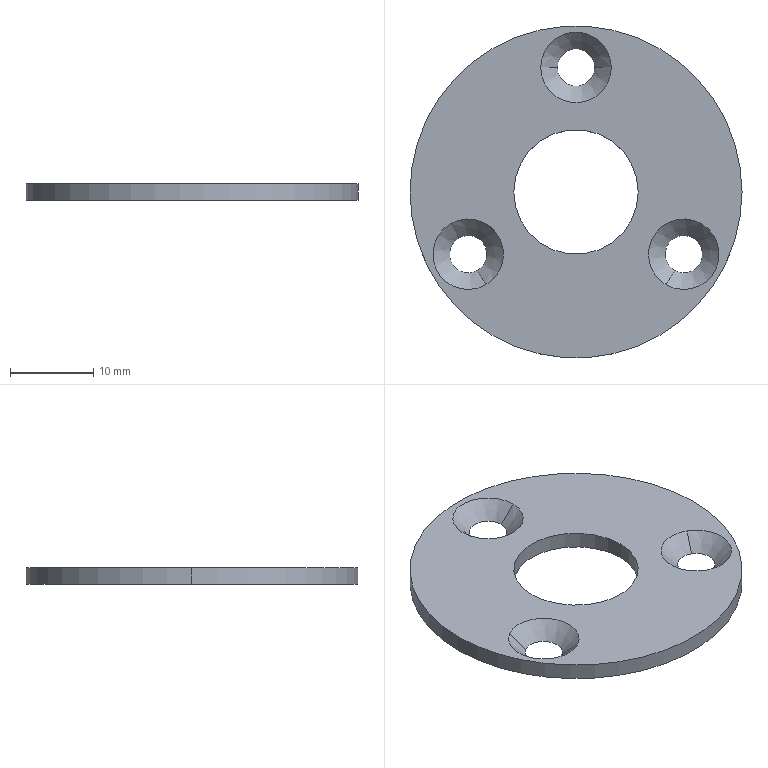Part | SolidWorks | features CirPattern 1, RevCut 1, Revolution 1 | 1 solid | 12 faces | box 40 x 40 x 2 mm | volume 1954 mm3 | cone 6 | cylinder 4 | plane 2 | commonest cylinder face diameters 15 x2 40 x2
STEP:
#1=CARTESIAN_POINT('',(-11.865,-9.449,-2.));
#2=VERTEX_POINT('',#1);
#3=CARTESIAN_POINT('',(-14.115,-5.551,-2.));
#4=VERTEX_POINT('',#3);
#5=CARTESIAN_POINT('',(-12.99,-7.5,-2.));
#6=DIRECTION('',(0.,0.,1.));
#7=DIRECTION('',(-0.5,0.866,0.));
#8=AXIS2_PLACEMENT_3D('',#5,#6,#7);
#9=CIRCLE('',#8,2.25);
#10=EDGE_CURVE('',#2,#4,#9,.T.);
#11=ORIENTED_EDGE('',*,*,#10,.F.);
#12=CARTESIAN_POINT('',(-10.865,-11.181,0.));
#13=VERTEX_POINT('',#12);
#14=CARTESIAN_POINT('',(-11.865,-9.449,-2.));
#15=DIRECTION('',(0.3536,-0.6124,0.7071));
#16=VECTOR('',#15,1000.);
#17=LINE('',#14,#16);
#18=EDGE_CURVE('',#2,#13,#17,.T.);
#19=ORIENTED_EDGE('',*,*,#18,.T.);
#20=CARTESIAN_POINT('',(-15.115,-3.819,0.));
#21=VERTEX_POINT('',#20);
#22=CARTESIAN_POINT('',(-12.99,-7.5,0.));
#23=DIRECTION('',(0.,0.,1.));
#24=DIRECTION('',(-0.5,0.866,0.));
#25=AXIS2_PLACEMENT_3D('',#22,#23,#24);
#26=CIRCLE('',#25,4.25);
#27=EDGE_CURVE('',#13,#21,#26,.T.);
#28=ORIENTED_EDGE('',*,*,#27,.T.);
#29=CARTESIAN_POINT('',(-14.115,-5.551,-2.));
#30=DIRECTION('',(-0.3536,0.6124,0.7071));
#31=VECTOR('',#30,1000.);
#32=LINE('',#29,#31);
#33=EDGE_CURVE('',#4,#21,#32,.T.);
#34=ORIENTED_EDGE('',*,*,#33,.F.);
#35=EDGE_LOOP('',(#11,#19,#28,#34));
#36=FACE_OUTER_BOUND('',#35,.T.);
#37=CARTESIAN_POINT('',(-12.99,-7.5,-2.));
#38=DIRECTION('',(0.,0.,1.));
#39=DIRECTION('',(-0.5,0.866,0.));
#40=AXIS2_PLACEMENT_3D('',#37,#38,#39);
#41=CONICAL_SURFACE('',#40,2.25,0.7854);
#42=ADVANCED_FACE('',(#36),#41,.F.);
#43=CARTESIAN_POINT('',(14.115,-5.551,-2.));
#44=VERTEX_POINT('',#43);
#45=CARTESIAN_POINT('',(11.865,-9.449,-2.));
#46=VERTEX_POINT('',#45);
#47=CARTESIAN_POINT('',(12.99,-7.5,-2.));
#48=DIRECTION('',(0.,0.,1.));
#49=DIRECTION('',(-0.5,-0.866,0.));
#50=AXIS2_PLACEMENT_3D('',#47,#48,#49);
#51=CIRCLE('',#50,2.25);
#52=EDGE_CURVE('',#44,#46,#51,.T.);
#53=ORIENTED_EDGE('',*,*,#52,.F.);
#54=CARTESIAN_POINT('',(15.115,-3.819,0.));
#55=VERTEX_POINT('',#54);
#56=CARTESIAN_POINT('',(14.115,-5.551,-2.));
#57=DIRECTION('',(0.3536,0.6124,0.7071));
#58=VECTOR('',#57,1000.);
#59=LINE('',#56,#58);
#60=EDGE_CURVE('',#44,#55,#59,.T.);
#61=ORIENTED_EDGE('',*,*,#60,.T.);
#62=CARTESIAN_POINT('',(10.865,-11.181,0.));
#63=VERTEX_POINT('',#62);
#64=CARTESIAN_POINT('',(12.99,-7.5,0.));
#65=DIRECTION('',(0.,0.,1.));
#66=DIRECTION('',(-0.5,-0.866,0.));
#67=AXIS2_PLACEMENT_3D('',#64,#65,#66);
#68=CIRCLE('',#67,4.25);
#69=EDGE_CURVE('',#55,#63,#68,.T.);
#70=ORIENTED_EDGE('',*,*,#69,.T.);
#71=CARTESIAN_POINT('',(11.865,-9.449,-2.));
#72=DIRECTION('',(-0.3536,-0.6124,0.7071));
#73=VECTOR('',#72,1000.);
#74=LINE('',#71,#73);
#75=EDGE_CURVE('',#46,#63,#74,.T.);
#76=ORIENTED_EDGE('',*,*,#75,.F.);
#77=EDGE_LOOP('',(#53,#61,#70,#76));
#78=FACE_OUTER_BOUND('',#77,.T.);
#79=CARTESIAN_POINT('',(12.99,-7.5,-2.));
#80=DIRECTION('',(0.,0.,1.));
#81=DIRECTION('',(-0.5,-0.866,0.));
#82=AXIS2_PLACEMENT_3D('',#79,#80,#81);
#83=CONICAL_SURFACE('',#82,2.25,0.7854);
#84=ADVANCED_FACE('',(#78),#83,.F.);
#85=CARTESIAN_POINT('',(-2.25,15.,-2.));
#86=VERTEX_POINT('',#85);
#87=CARTESIAN_POINT('',(2.25,15.,-2.));
#88=VERTEX_POINT('',#87);
#89=CARTESIAN_POINT('',(0.,15.,-2.));
#90=DIRECTION('',(0.,0.,1.));
#91=DIRECTION('',(1.,0.,0.));
#92=AXIS2_PLACEMENT_3D('',#89,#90,#91);
#93=CIRCLE('',#92,2.25);
#94=EDGE_CURVE('',#86,#88,#93,.T.);
#95=ORIENTED_EDGE('',*,*,#94,.F.);
#96=CARTESIAN_POINT('',(-4.25,15.,0.));
#97=VERTEX_POINT('',#96);
#98=CARTESIAN_POINT('',(-2.25,15.,-2.));
#99=DIRECTION('',(-0.7071,0.,0.7071));
#100=VECTOR('',#99,1000.);
#101=LINE('',#98,#100);
#102=EDGE_CURVE('',#86,#97,#101,.T.);
#103=ORIENTED_EDGE('',*,*,#102,.T.);
#104=CARTESIAN_POINT('',(4.25,15.,0.));
#105=VERTEX_POINT('',#104);
#106=CARTESIAN_POINT('',(0.,15.,0.));
#107=DIRECTION('',(0.,0.,1.));
#108=DIRECTION('',(1.,0.,0.));
#109=AXIS2_PLACEMENT_3D('',#106,#107,#108);
#110=CIRCLE('',#109,4.25);
#111=EDGE_CURVE('',#97,#105,#110,.T.);
#112=ORIENTED_EDGE('',*,*,#111,.T.);
#113=CARTESIAN_POINT('',(2.25,15.,-2.));
#114=DIRECTION('',(0.7071,0.,0.7071));
#115=VECTOR('',#114,1000.);
#116=LINE('',#113,#115);
#117=EDGE_CURVE('',#88,#105,#116,.T.);
#118=ORIENTED_EDGE('',*,*,#117,.F.);
#119=EDGE_LOOP('',(#95,#103,#112,#118));
#120=FACE_OUTER_BOUND('',#119,.T.);
#121=CARTESIAN_POINT('',(0.,15.,-2.));
#122=DIRECTION('',(0.,0.,1.));
#123=DIRECTION('',(1.,0.,0.));
#124=AXIS2_PLACEMENT_3D('',#121,#122,#123);
#125=CONICAL_SURFACE('',#124,2.25,0.7854);
#126=ADVANCED_FACE('',(#120),#125,.F.);
#127=CARTESIAN_POINT('',(-7.5,0.,-2.));
#128=VERTEX_POINT('',#127);
#129=CARTESIAN_POINT('',(7.5,0.,-2.));
#130=VERTEX_POINT('',#129);
#131=CARTESIAN_POINT('',(0.,0.,-2.));
#132=DIRECTION('',(0.,0.,1.));
#133=DIRECTION('',(1.,0.,0.));
#134=AXIS2_PLACEMENT_3D('',#131,#132,#133);
#135=CIRCLE('',#134,7.5);
#136=EDGE_CURVE('',#128,#130,#135,.T.);
#137=ORIENTED_EDGE('',*,*,#136,.F.);
#138=CARTESIAN_POINT('',(-7.5,0.,0.));
#139=VERTEX_POINT('',#138);
#140=CARTESIAN_POINT('',(-7.5,0.,4.367));
#141=DIRECTION('',(0.,0.,1.));
#142=VECTOR('',#141,1000.);
#143=LINE('',#140,#142);
#144=EDGE_CURVE('',#128,#139,#143,.T.);
#145=ORIENTED_EDGE('',*,*,#144,.T.);
#146=CARTESIAN_POINT('',(7.5,0.,0.));
#147=VERTEX_POINT('',#146);
#148=CARTESIAN_POINT('',(0.,0.,0.));
#149=DIRECTION('',(0.,0.,1.));
#150=DIRECTION('',(1.,0.,0.));
#151=AXIS2_PLACEMENT_3D('',#148,#149,#150);
#152=CIRCLE('',#151,7.5);
#153=EDGE_CURVE('',#139,#147,#152,.T.);
#154=ORIENTED_EDGE('',*,*,#153,.T.);
#155=CARTESIAN_POINT('',(7.5,0.,4.367));
#156=DIRECTION('',(0.,0.,1.));
#157=VECTOR('',#156,1000.);
#158=LINE('',#155,#157);
#159=EDGE_CURVE('',#130,#147,#158,.T.);
#160=ORIENTED_EDGE('',*,*,#159,.F.);
#161=EDGE_LOOP('',(#137,#145,#154,#160));
#162=FACE_OUTER_BOUND('',#161,.T.);
#163=CARTESIAN_POINT('',(0.,0.,4.367));
#164=DIRECTION('',(0.,0.,1.));
#165=DIRECTION('',(1.,0.,0.));
#166=AXIS2_PLACEMENT_3D('',#163,#164,#165);
#167=CYLINDRICAL_SURFACE('',#166,7.5);
#168=ADVANCED_FACE('',(#162),#167,.F.);
#169=CARTESIAN_POINT('',(20.,0.,-2.));
#170=VERTEX_POINT('',#169);
#171=CARTESIAN_POINT('',(-20.,0.,-2.));
#172=VERTEX_POINT('',#171);
#173=CARTESIAN_POINT('',(0.,0.,-2.));
#174=DIRECTION('',(0.,0.,1.));
#175=DIRECTION('',(1.,0.,0.));
#176=AXIS2_PLACEMENT_3D('',#173,#174,#175);
#177=CIRCLE('',#176,20.);
#178=EDGE_CURVE('',#170,#172,#177,.T.);
#179=ORIENTED_EDGE('',*,*,#178,.T.);
#180=CARTESIAN_POINT('',(-20.,0.,0.));
#181=VERTEX_POINT('',#180);
#182=CARTESIAN_POINT('',(-20.,0.,4.367));
#183=DIRECTION('',(0.,0.,1.));
#184=VECTOR('',#183,1000.);
#185=LINE('',#182,#184);
#186=EDGE_CURVE('',#172,#181,#185,.T.);
#187=ORIENTED_EDGE('',*,*,#186,.T.);
#188=CARTESIAN_POINT('',(20.,0.,0.));
#189=VERTEX_POINT('',#188);
#190=CARTESIAN_POINT('',(0.,0.,0.));
#191=DIRECTION('',(0.,0.,1.));
#192=DIRECTION('',(1.,0.,0.));
#193=AXIS2_PLACEMENT_3D('',#190,#191,#192);
#194=CIRCLE('',#193,20.);
#195=EDGE_CURVE('',#189,#181,#194,.T.);
#196=ORIENTED_EDGE('',*,*,#195,.F.);
#197=CARTESIAN_POINT('',(20.,0.,4.367));
#198=DIRECTION('',(0.,0.,1.));
#199=VECTOR('',#198,1000.);
#200=LINE('',#197,#199);
#201=EDGE_CURVE('',#170,#189,#200,.T.);
#202=ORIENTED_EDGE('',*,*,#201,.F.);
#203=EDGE_LOOP('',(#179,#187,#196,#202));
#204=FACE_OUTER_BOUND('',#203,.T.);
#205=CARTESIAN_POINT('',(0.,0.,4.367));
#206=DIRECTION('',(0.,0.,1.));
#207=DIRECTION('',(1.,0.,0.));
#208=AXIS2_PLACEMENT_3D('',#205,#206,#207);
#209=CYLINDRICAL_SURFACE('',#208,20.);
#210=ADVANCED_FACE('',(#204),#209,.T.);
#211=ORIENTED_EDGE('',*,*,#186,.F.);
#212=CARTESIAN_POINT('',(0.,0.,-2.));
#213=DIRECTION('',(0.,0.,1.));
#214=DIRECTION('',(1.,0.,0.));
#215=AXIS2_PLACEMENT_3D('',#212,#213,#214);
#216=CIRCLE('',#215,20.);
#217=EDGE_CURVE('',#172,#170,#216,.T.);
#218=ORIENTED_EDGE('',*,*,#217,.T.);
#219=ORIENTED_EDGE('',*,*,#201,.T.);
#220=CARTESIAN_POINT('',(0.,0.,0.));
#221=DIRECTION('',(0.,0.,1.));
#222=DIRECTION('',(1.,0.,0.));
#223=AXIS2_PLACEMENT_3D('',#220,#221,#222);
#224=CIRCLE('',#223,20.);
#225=EDGE_CURVE('',#181,#189,#224,.T.);
#226=ORIENTED_EDGE('',*,*,#225,.F.);
#227=EDGE_LOOP('',(#211,#218,#219,#226));
#228=FACE_OUTER_BOUND('',#227,.T.);
#229=CARTESIAN_POINT('',(0.,0.,4.367));
#230=DIRECTION('',(0.,0.,1.));
#231=DIRECTION('',(1.,0.,0.));
#232=AXIS2_PLACEMENT_3D('',#229,#230,#231);
#233=CYLINDRICAL_SURFACE('',#232,20.);
#234=ADVANCED_FACE('',(#228),#233,.T.);
#235=CARTESIAN_POINT('',(-12.99,-7.5,0.));
#236=DIRECTION('',(0.,0.,1.));
#237=DIRECTION('',(-0.5,0.866,0.));
#238=AXIS2_PLACEMENT_3D('',#235,#236,#237);
#239=CIRCLE('',#238,4.25);
#240=EDGE_CURVE('',#21,#13,#239,.T.);
#241=ORIENTED_EDGE('',*,*,#240,.F.);
#242=ORIENTED_EDGE('',*,*,#27,.F.);
#243=EDGE_LOOP('',(#241,#242));
#244=FACE_BOUND('',#243,.T.);
#245=CARTESIAN_POINT('',(12.99,-7.5,0.));
#246=DIRECTION('',(0.,0.,1.));
#247=DIRECTION('',(-0.5,-0.866,0.));
#248=AXIS2_PLACEMENT_3D('',#245,#246,#247);
#249=CIRCLE('',#248,4.25);
#250=EDGE_CURVE('',#63,#55,#249,.T.);
#251=ORIENTED_EDGE('',*,*,#250,.F.);
#252=ORIENTED_EDGE('',*,*,#69,.F.);
#253=EDGE_LOOP('',(#251,#252));
#254=FACE_BOUND('',#253,.T.);
#255=CARTESIAN_POINT('',(0.,15.,0.));
#256=DIRECTION('',(0.,0.,1.));
#257=DIRECTION('',(1.,0.,0.));
#258=AXIS2_PLACEMENT_3D('',#255,#256,#257);
#259=CIRCLE('',#258,4.25);
#260=EDGE_CURVE('',#105,#97,#259,.T.);
#261=ORIENTED_EDGE('',*,*,#260,.F.);
#262=ORIENTED_EDGE('',*,*,#111,.F.);
#263=EDGE_LOOP('',(#261,#262));
#264=FACE_BOUND('',#263,.T.);
#265=CARTESIAN_POINT('',(0.,0.,0.));
#266=DIRECTION('',(0.,0.,1.));
#267=DIRECTION('',(1.,0.,0.));
#268=AXIS2_PLACEMENT_3D('',#265,#266,#267);
#269=CIRCLE('',#268,7.5);
#270=EDGE_CURVE('',#147,#139,#269,.T.);
#271=ORIENTED_EDGE('',*,*,#270,.F.);
#272=ORIENTED_EDGE('',*,*,#153,.F.);
#273=EDGE_LOOP('',(#271,#272));
#274=FACE_BOUND('',#273,.T.);
#275=ORIENTED_EDGE('',*,*,#195,.T.);
#276=ORIENTED_EDGE('',*,*,#225,.T.);
#277=EDGE_LOOP('',(#275,#276));
#278=FACE_OUTER_BOUND('',#277,.T.);
#279=CARTESIAN_POINT('',(0.,20.,0.));
#280=DIRECTION('',(0.,0.,-1.));
#281=DIRECTION('',(-1.,0.,0.));
#282=AXIS2_PLACEMENT_3D('',#279,#280,#281);
#283=PLANE('',#282);
#284=ADVANCED_FACE('',(#244,#254,#264,#274,#278),#283,.F.);
#285=ORIENTED_EDGE('',*,*,#144,.F.);
#286=CARTESIAN_POINT('',(0.,0.,-2.));
#287=DIRECTION('',(0.,0.,1.));
#288=DIRECTION('',(1.,0.,0.));
#289=AXIS2_PLACEMENT_3D('',#286,#287,#288);
#290=CIRCLE('',#289,7.5);
#291=EDGE_CURVE('',#130,#128,#290,.T.);
#292=ORIENTED_EDGE('',*,*,#291,.F.);
#293=ORIENTED_EDGE('',*,*,#159,.T.);
#294=ORIENTED_EDGE('',*,*,#270,.T.);
#295=EDGE_LOOP('',(#285,#292,#293,#294));
#296=FACE_OUTER_BOUND('',#295,.T.);
#297=CARTESIAN_POINT('',(0.,0.,4.367));
#298=DIRECTION('',(0.,0.,1.));
#299=DIRECTION('',(1.,0.,0.));
#300=AXIS2_PLACEMENT_3D('',#297,#298,#299);
#301=CYLINDRICAL_SURFACE('',#300,7.5);
#302=ADVANCED_FACE('',(#296),#301,.F.);
#303=CARTESIAN_POINT('',(-12.99,-7.5,-2.));
#304=DIRECTION('',(0.,0.,1.));
#305=DIRECTION('',(-0.5,0.866,0.));
#306=AXIS2_PLACEMENT_3D('',#303,#304,#305);
#307=CIRCLE('',#306,2.25);
#308=EDGE_CURVE('',#4,#2,#307,.T.);
#309=ORIENTED_EDGE('',*,*,#308,.T.);
#310=ORIENTED_EDGE('',*,*,#10,.T.);
#311=EDGE_LOOP('',(#309,#310));
#312=FACE_BOUND('',#311,.T.);
#313=CARTESIAN_POINT('',(12.99,-7.5,-2.));
#314=DIRECTION('',(0.,0.,1.));
#315=DIRECTION('',(-0.5,-0.866,0.));
#316=AXIS2_PLACEMENT_3D('',#313,#314,#315);
#317=CIRCLE('',#316,2.25);
#318=EDGE_CURVE('',#46,#44,#317,.T.);
#319=ORIENTED_EDGE('',*,*,#318,.T.);
#320=ORIENTED_EDGE('',*,*,#52,.T.);
#321=EDGE_LOOP('',(#319,#320));
#322=FACE_BOUND('',#321,.T.);
#323=CARTESIAN_POINT('',(0.,15.,-2.));
#324=DIRECTION('',(0.,0.,1.));
#325=DIRECTION('',(1.,0.,0.));
#326=AXIS2_PLACEMENT_3D('',#323,#324,#325);
#327=CIRCLE('',#326,2.25);
#328=EDGE_CURVE('',#88,#86,#327,.T.);
#329=ORIENTED_EDGE('',*,*,#328,.T.);
#330=ORIENTED_EDGE('',*,*,#94,.T.);
#331=EDGE_LOOP('',(#329,#330));
#332=FACE_BOUND('',#331,.T.);
#333=ORIENTED_EDGE('',*,*,#178,.F.);
#334=ORIENTED_EDGE('',*,*,#217,.F.);
#335=EDGE_LOOP('',(#333,#334));
#336=FACE_OUTER_BOUND('',#335,.T.);
#337=ORIENTED_EDGE('',*,*,#291,.T.);
#338=ORIENTED_EDGE('',*,*,#136,.T.);
#339=EDGE_LOOP('',(#337,#338));
#340=FACE_BOUND('',#339,.T.);
#341=CARTESIAN_POINT('',(0.,7.5,-2.));
#342=DIRECTION('',(0.,0.,1.));
#343=DIRECTION('',(1.,0.,0.));
#344=AXIS2_PLACEMENT_3D('',#341,#342,#343);
#345=PLANE('',#344);
#346=ADVANCED_FACE('',(#312,#322,#332,#336,#340),#345,.F.);
#347=ORIENTED_EDGE('',*,*,#102,.F.);
#348=ORIENTED_EDGE('',*,*,#328,.F.);
#349=ORIENTED_EDGE('',*,*,#117,.T.);
#350=ORIENTED_EDGE('',*,*,#260,.T.);
#351=EDGE_LOOP('',(#347,#348,#349,#350));
#352=FACE_OUTER_BOUND('',#351,.T.);
#353=CARTESIAN_POINT('',(0.,15.,-2.));
#354=DIRECTION('',(0.,0.,1.));
#355=DIRECTION('',(1.,0.,0.));
#356=AXIS2_PLACEMENT_3D('',#353,#354,#355);
#357=CONICAL_SURFACE('',#356,2.25,0.7854);
#358=ADVANCED_FACE('',(#352),#357,.F.);
#359=ORIENTED_EDGE('',*,*,#60,.F.);
#360=ORIENTED_EDGE('',*,*,#318,.F.);
#361=ORIENTED_EDGE('',*,*,#75,.T.);
#362=ORIENTED_EDGE('',*,*,#250,.T.);
#363=EDGE_LOOP('',(#359,#360,#361,#362));
#364=FACE_OUTER_BOUND('',#363,.T.);
#365=CARTESIAN_POINT('',(12.99,-7.5,-2.));
#366=DIRECTION('',(0.,0.,1.));
#367=DIRECTION('',(-0.5,-0.866,0.));
#368=AXIS2_PLACEMENT_3D('',#365,#366,#367);
#369=CONICAL_SURFACE('',#368,2.25,0.7854);
#370=ADVANCED_FACE('',(#364),#369,.F.);
#371=ORIENTED_EDGE('',*,*,#18,.F.);
#372=ORIENTED_EDGE('',*,*,#308,.F.);
#373=ORIENTED_EDGE('',*,*,#33,.T.);
#374=ORIENTED_EDGE('',*,*,#240,.T.);
#375=EDGE_LOOP('',(#371,#372,#373,#374));
#376=FACE_OUTER_BOUND('',#375,.T.);
#377=CARTESIAN_POINT('',(-12.99,-7.5,-2.));
#378=DIRECTION('',(0.,0.,1.));
#379=DIRECTION('',(-0.5,0.866,0.));
#380=AXIS2_PLACEMENT_3D('',#377,#378,#379);
#381=CONICAL_SURFACE('',#380,2.25,0.7854);
#382=ADVANCED_FACE('',(#376),#381,.F.);
#383=CLOSED_SHELL('',(#42,#84,#126,#168,#210,#234,#284,#302,#346,#358,#370,#382));
#384=MANIFOLD_SOLID_BREP('',#383);
#385=CARTESIAN_POINT('',(0.,0.,0.));
#386=DIRECTION('',(0.,0.,1.));
#387=DIRECTION('',(1.,0.,0.));
#388=AXIS2_PLACEMENT_3D('',#385,#386,#387);
#389=(LENGTH_UNIT()NAMED_UNIT(*)SI_UNIT(.MILLI.,.METRE.));
#390=UNCERTAINTY_MEASURE_WITH_UNIT(LENGTH_MEASURE(0.00001),#389,'','');
#391=(NAMED_UNIT(*)PLANE_ANGLE_UNIT()SI_UNIT($,.RADIAN.));
#392=(NAMED_UNIT(*)SI_UNIT($,.STERADIAN.)SOLID_ANGLE_UNIT());
#393=(GEOMETRIC_REPRESENTATION_CONTEXT(3)GLOBAL_UNCERTAINTY_ASSIGNED_CONTEXT((#390))GLOBAL_UNIT_ASSIGNED_CONTEXT((#389,#391,#392))REPRESENTATION_CONTEXT('',''));
#394=ADVANCED_BREP_SHAPE_REPRESENTATION('',(#384,#388),#393);